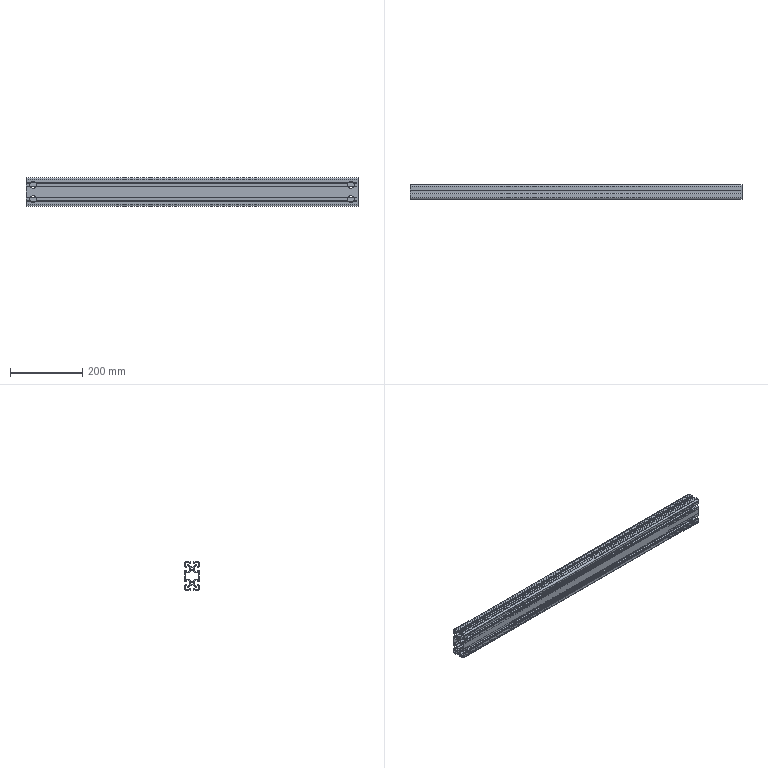Part | STEP file | Aluminum Profile | 1 solid | 550 faces | box 920 x 40 x 80 mm | volume 738290 mm3 | cylinder 296 | plane 254 | commonest cylinder face diameters 0.6 x100 2 x60 4 x44 19 x40 0.4 x34 0.458 x6